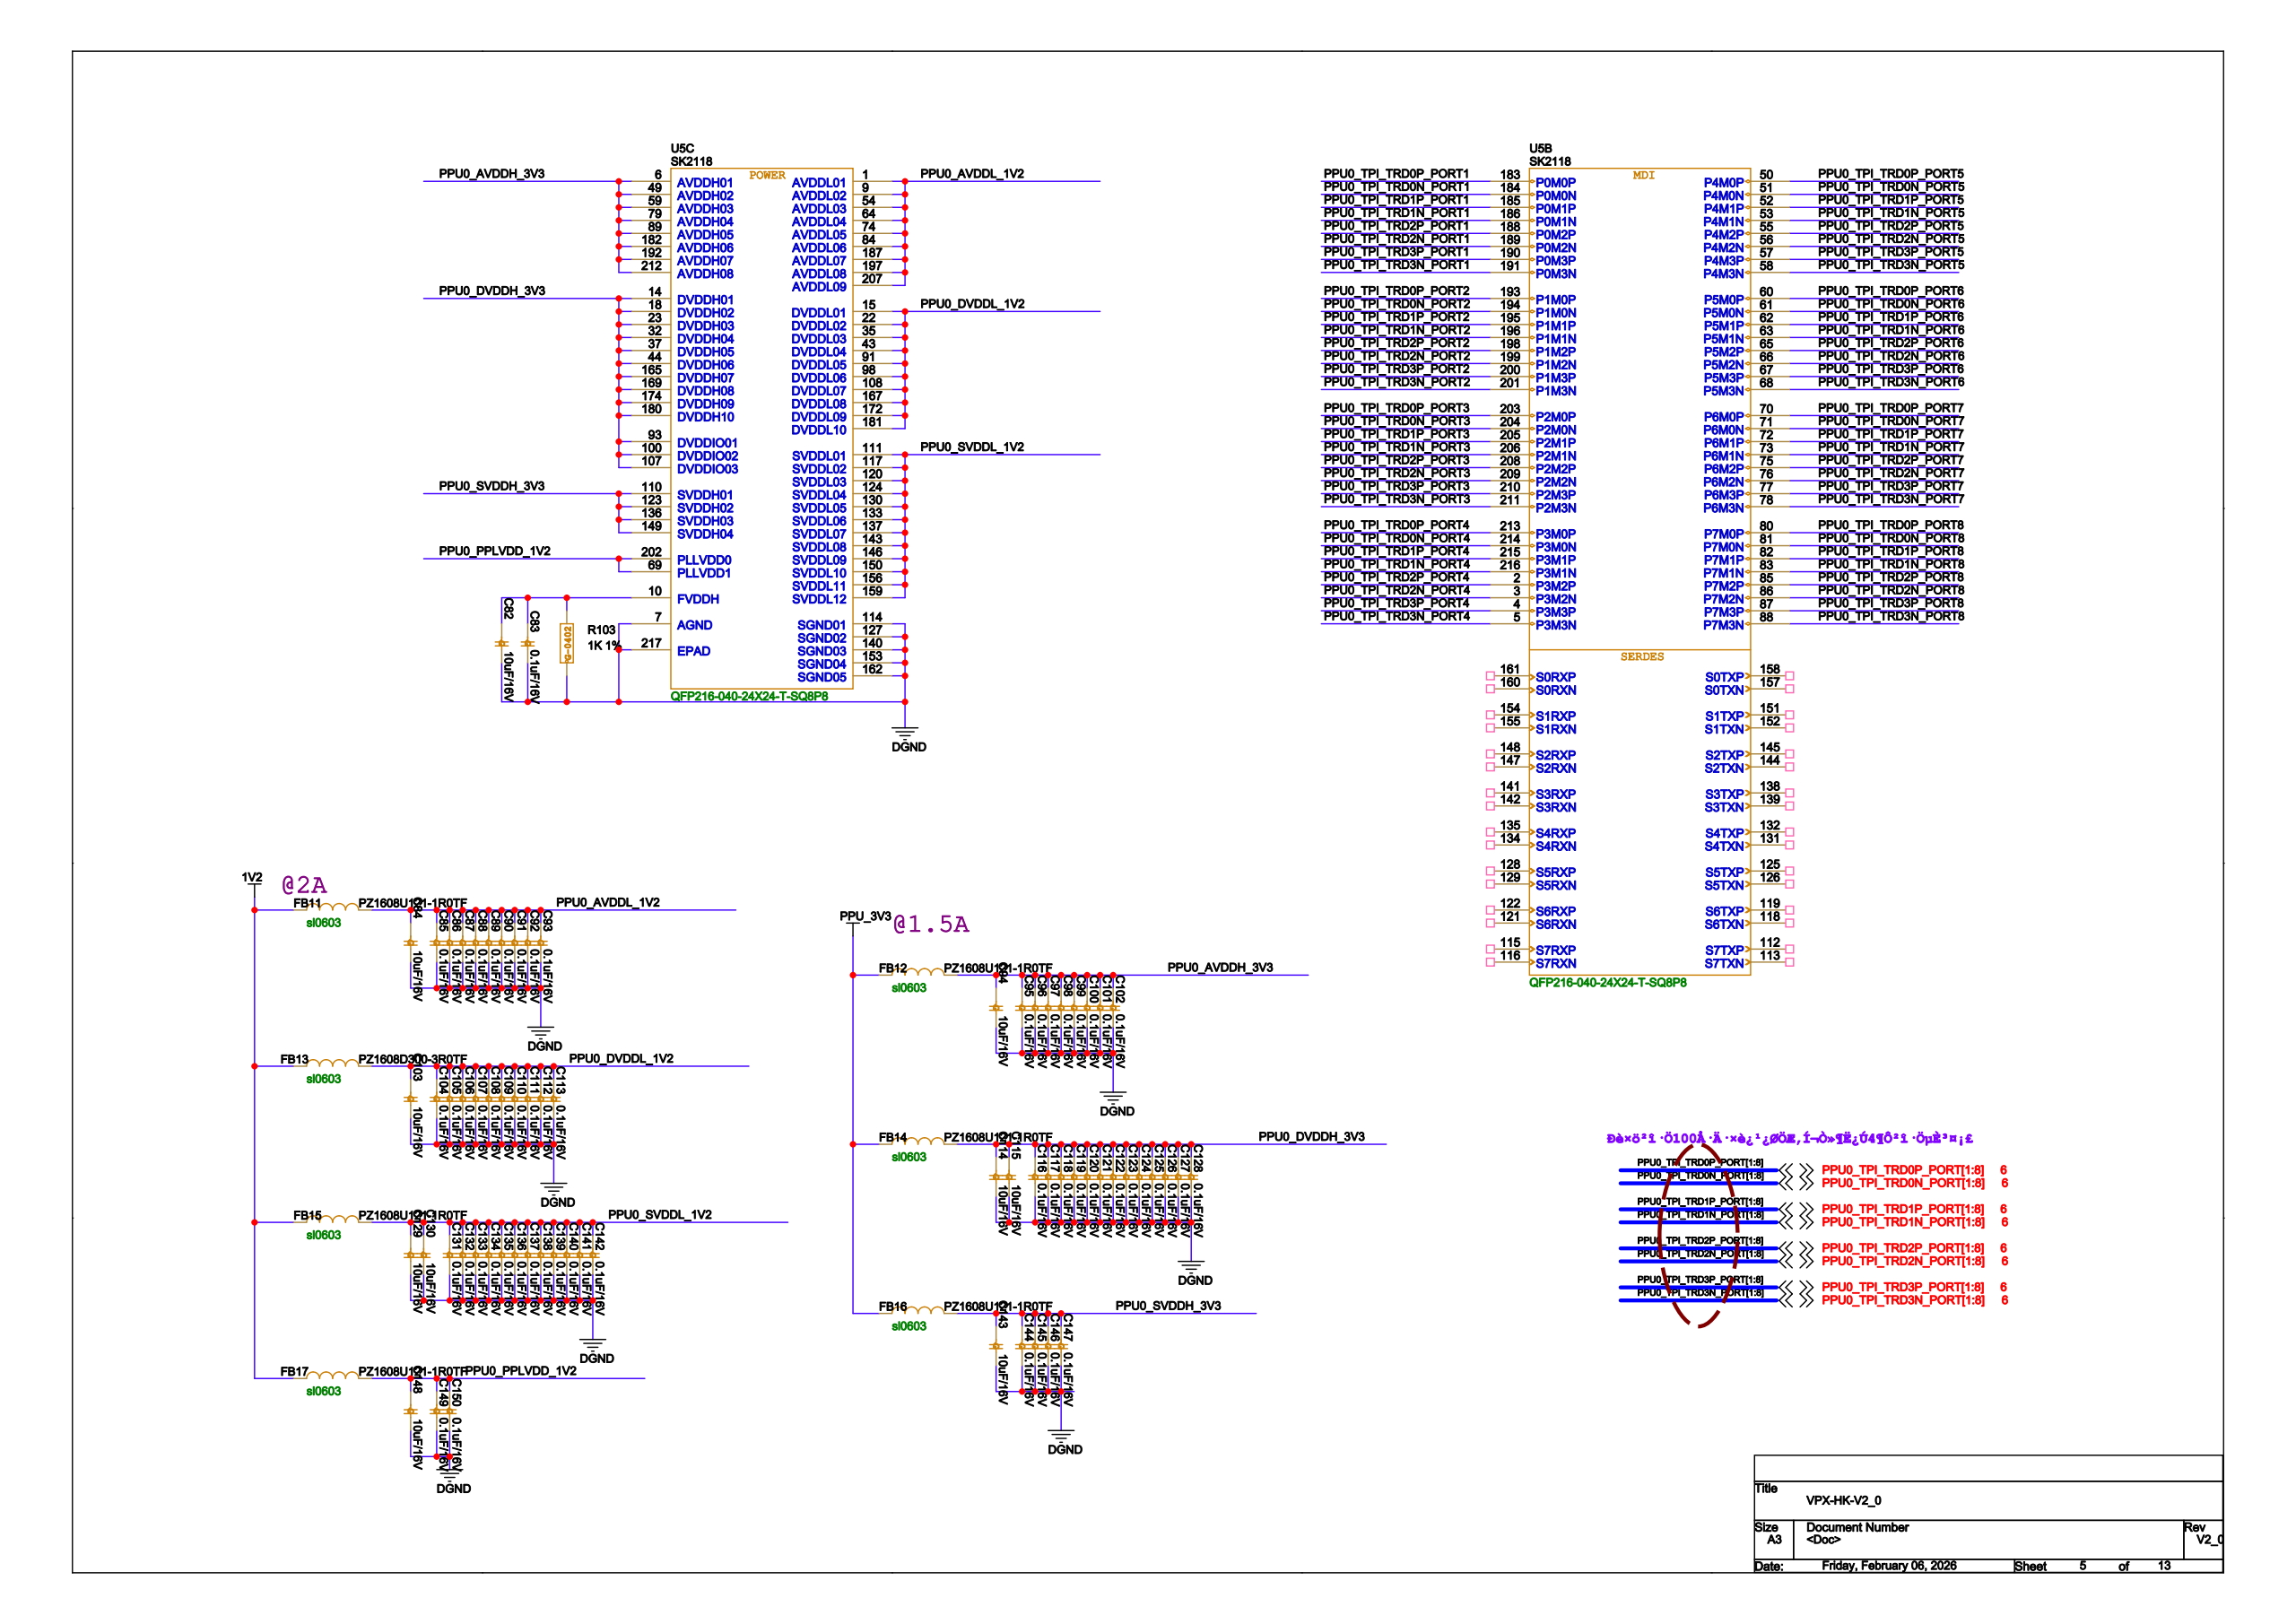Circuit board | Cadence Allegro | 598 parts | 541 nets | one sheet of the schematic
Parts on this sheet (reference | value | footprint):
C82 | 10uF/16V | SC0603
C83 | 0.1uF/16V | SC0402
C84 | 10uF/16V | SC0603
C85 | 0.1uF/16V | SC0402
C86 | 0.1uF/16V | SC0402
C87 | 0.1uF/16V | SC0402
C88 | 0.1uF/16V | SC0402
C89 | 0.1uF/16V | SC0402
C90 | 0.1uF/16V | SC0402
C91 | 0.1uF/16V | SC0402
C92 | 0.1uF/16V | SC0402
C93 | 0.1uF/16V | SC0402
C94 | 10uF/16V | SC0603
C95 | 0.1uF/16V | SC0402
C96 | 0.1uF/16V | SC0402
C97 | 0.1uF/16V | SC0402
C98 | 0.1uF/16V | SC0402
C99 | 0.1uF/16V | SC0402
C100 | 0.1uF/16V | SC0402
C101 | 0.1uF/16V | SC0402
C102 | 0.1uF/16V | SC0402
C103 | 10uF/16V | SC0603
C104 | 0.1uF/16V | SC0402
C105 | 0.1uF/16V | SC0402
C106 | 0.1uF/16V | SC0402
C107 | 0.1uF/16V | SC0402
C108 | 0.1uF/16V | SC0402
C109 | 0.1uF/16V | SC0402
C110 | 0.1uF/16V | SC0402
C111 | 0.1uF/16V | SC0402
C112 | 0.1uF/16V | SC0402
C113 | 0.1uF/16V | SC0402
C114 | 10uF/16V | SC0603
C115 | 10uF/16V | SC0603
C116 | 0.1uF/16V | SC0402
C117 | 0.1uF/16V | SC0402
C118 | 0.1uF/16V | SC0402
C119 | 0.1uF/16V | SC0402
C120 | 0.1uF/16V | SC0402
C121 | 0.1uF/16V | SC0402
C122 | 0.1uF/16V | SC0402
C123 | 0.1uF/16V | SC0402
C124 | 0.1uF/16V | SC0402
C125 | 0.1uF/16V | SC0402
C126 | 0.1uF/16V | SC0402
C127 | 0.1uF/16V | SC0402
C128 | 0.1uF/16V | SC0402
C129 | 10uF/16V | SC0603
C130 | 10uF/16V | SC0603
C131 | 0.1uF/16V | SC0402
C132 | 0.1uF/16V | SC0402
C133 | 0.1uF/16V | SC0402
C134 | 0.1uF/16V | SC0402
C135 | 0.1uF/16V | SC0402
C136 | 0.1uF/16V | SC0402
C137 | 0.1uF/16V | SC0402
C138 | 0.1uF/16V | SC0402
C139 | 0.1uF/16V | SC0402
C140 | 0.1uF/16V | SC0402
C141 | 0.1uF/16V | SC0402
C142 | 0.1uF/16V | SC0402
C143 | 10uF/16V | SC0603
C144 | 0.1uF/16V | SC0402
C145 | 0.1uF/16V | SC0402
C146 | 0.1uF/16V | SC0402
C147 | 0.1uF/16V | SC0402
C148 | 10uF/16V | SC0603
C149 | 0.1uF/16V | SC0402
C150 | 0.1uF/16V | SC0402
FB11 | PZ1608U121-1R0TF | SL0603
FB12 | PZ1608U121-1R0TF | SL0603
FB13 | PZ1608D300-3R0TF | SL0603
FB14 | PZ1608U121-1R0TF | SL0603
FB15 | PZ1608U121-1R0TF | SL0603
FB16 | PZ1608U121-1R0TF | SL0603
FB17 | PZ1608U121-1R0TF | SL0603
R103 | 1K 1% | SR0402
U5 | SK2118 | QFP216-040-24X24-T-SQ8P8
Nets of these parts (net: part-pin ...):
1V2: FB11-1 FB13-1 FB15-1 FB17-1
PPU_3V3: FB12-1 FB14-1 FB16-1
DGND: C82-2 C83-2 C84-2 C85-2 C86-2 C87-2 C88-2 C89-2 C90-2 C91-2 C92-2 C93-2 C94-2 C95-2 C96-2 C97-2 C98-2 C99-2 C100-2 C101-2 C102-2 C103-2 C104-2 C105-2 C106-2 C107-2 C108-2 C109-2 C110-2 C111-2 C112-2 C113-2 C114-2 C115-2 C116-2 C117-2 C118-2 C119-2 C120-2 C121-2 C122-2 C123-2 C124-2 C125-2 C126-2 C127-2 C128-2 C129-2 C130-2 C131-2 C132-2 C133-2 C134-2 C135-2 C136-2 C137-2 C138-2 C139-2 C140-2 C141-2 C142-2 C143-2 C144-2 C145-2 C146-2 C147-2 C148-2 C149-2 C150-2 R103-1 U5-7 U5-114 U5-127 U5-140 U5-153 U5-162 U5-217
PPU0_AVDDL_1V2: C84-1 C85-1 C86-1 C87-1 C88-1 C89-1 C90-1 C91-1 C92-1 C93-1 FB11-2 U5-1 U5-9 U5-54 U5-64 U5-74 U5-84 U5-187 U5-197 U5-207
PPU0_AVDDH_3V3: C94-1 C95-1 C96-1 C97-1 C98-1 C99-1 C100-1 C101-1 C102-1 FB12-2 U5-6 U5-49 U5-59 U5-79 U5-89 U5-182 U5-192 U5-212
PPU0_DVDDH_3V3: C114-1 C115-1 C116-1 C117-1 C118-1 C119-1 C120-1 C121-1 C122-1 C123-1 C124-1 C125-1 C126-1 C127-1 C128-1 FB14-2 U5-14 U5-18 U5-23 U5-32 U5-37 U5-44 U5-93 U5-100 U5-107 U5-165 U5-169 U5-174 U5-180
PPU0_SVDDL_1V2: C129-1 C130-1 C131-1 C132-1 C133-1 C134-1 C135-1 C136-1 C137-1 C138-1 C139-1 C140-1 C141-1 C142-1 FB15-2 U5-111 U5-117 U5-120 U5-124 U5-130 U5-133 U5-137 U5-143 U5-146 U5-150 U5-156 U5-159
PPU0_SVDDH_3V3: C143-1 C144-1 C145-1 C146-1 C147-1 FB16-2 U5-110 U5-123 U5-136 U5-149
PPU0_PPLVDD_1V2: C148-1 C149-1 C150-1 FB17-2 U5-69 U5-202
PPU0_DVDDL_1V2: C103-1 C104-1 C105-1 C106-1 C107-1 C108-1 C109-1 C110-1 C111-1 C112-1 C113-1 FB13-2 U5-15 U5-22 U5-35 U5-43 U5-91 U5-98 U5-108 U5-167 U5-172 U5-181
N32903116: C82-1 C83-1 R103-2 U5-10
PPU0_TPI_TRD0N_PORT1: U5-184
PPU0_TPI_TRD0P_PORT1: U5-183
PPU0_TPI_TRD1N_PORT1: U5-186
PPU0_TPI_TRD1P_PORT1: U5-185
PPU0_TPI_TRD2N_PORT1: U5-189
PPU0_TPI_TRD2P_PORT1: U5-188
PPU0_TPI_TRD3N_PORT1: U5-191
PPU0_TPI_TRD3P_PORT1: U5-190
PPU0_TPI_TRD0N_PORT2: U5-194
PPU0_TPI_TRD0P_PORT2: U5-193
PPU0_TPI_TRD1N_PORT2: U5-196
PPU0_TPI_TRD1P_PORT2: U5-195
PPU0_TPI_TRD2N_PORT2: U5-199
PPU0_TPI_TRD2P_PORT2: U5-198
PPU0_TPI_TRD3N_PORT2: U5-201
PPU0_TPI_TRD3P_PORT2: U5-200
PPU0_TPI_TRD0N_PORT3: U5-204
PPU0_TPI_TRD0P_PORT3: U5-203
PPU0_TPI_TRD1N_PORT3: U5-206
PPU0_TPI_TRD1P_PORT3: U5-205
PPU0_TPI_TRD2N_PORT3: U5-209
PPU0_TPI_TRD2P_PORT3: U5-208
PPU0_TPI_TRD3N_PORT3: U5-211
PPU0_TPI_TRD3P_PORT3: U5-210
PPU0_TPI_TRD0N_PORT4: U5-214
PPU0_TPI_TRD0P_PORT4: U5-213
PPU0_TPI_TRD1N_PORT4: U5-216
PPU0_TPI_TRD1P_PORT4: U5-215
PPU0_TPI_TRD2N_PORT4: U5-3
PPU0_TPI_TRD2P_PORT4: U5-2
PPU0_TPI_TRD3N_PORT4: U5-5
PPU0_TPI_TRD3P_PORT4: U5-4
PPU0_TPI_TRD0N_PORT5: U5-51
PPU0_TPI_TRD0P_PORT5: U5-50
PPU0_TPI_TRD1N_PORT5: U5-53
PPU0_TPI_TRD1P_PORT5: U5-52
PPU0_TPI_TRD2N_PORT5: U5-56
PPU0_TPI_TRD2P_PORT5: U5-55
PPU0_TPI_TRD3N_PORT5: U5-58
PPU0_TPI_TRD3P_PORT5: U5-57
PPU0_TPI_TRD0N_PORT6: U5-61
PPU0_TPI_TRD0P_PORT6: U5-60
PPU0_TPI_TRD1N_PORT6: U5-63
PPU0_TPI_TRD1P_PORT6: U5-62
PPU0_TPI_TRD2N_PORT6: U5-66
PPU0_TPI_TRD2P_PORT6: U5-65
PPU0_TPI_TRD3N_PORT6: U5-68
PPU0_TPI_TRD3P_PORT6: U5-67
PPU0_TPI_TRD0N_PORT7: U5-71
PPU0_TPI_TRD0P_PORT7: U5-70
PPU0_TPI_TRD1N_PORT7: U5-73
PPU0_TPI_TRD1P_PORT7: U5-72
PPU0_TPI_TRD2N_PORT7: U5-76
PPU0_TPI_TRD2P_PORT7: U5-75
PPU0_TPI_TRD3N_PORT7: U5-78
PPU0_TPI_TRD3P_PORT7: U5-77
PPU0_TPI_TRD0N_PORT8: U5-81
PPU0_TPI_TRD0P_PORT8: U5-80
PPU0_TPI_TRD1N_PORT8: U5-83
PPU0_TPI_TRD1P_PORT8: U5-82
PPU0_TPI_TRD2N_PORT8: U5-86
PPU0_TPI_TRD2P_PORT8: U5-85
PPU0_TPI_TRD3N_PORT8: U5-88
PPU0_TPI_TRD3P_PORT8: U5-87